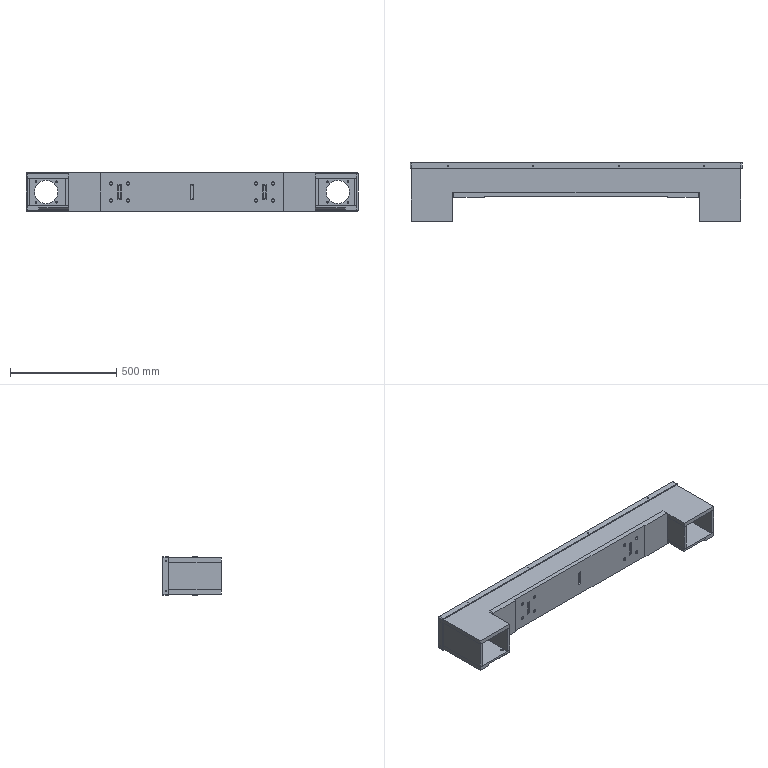Part | SolidWorks | 15 solids | 267 faces | box 1560 x 275 x 180 mm | volume 24061774 mm3 | plane 158 | cylinder 77 | cone 32 | commonest cylinder face diameters 14 x24 5 x16 8.5 x16 3 x9 10 x8 110.5 x4